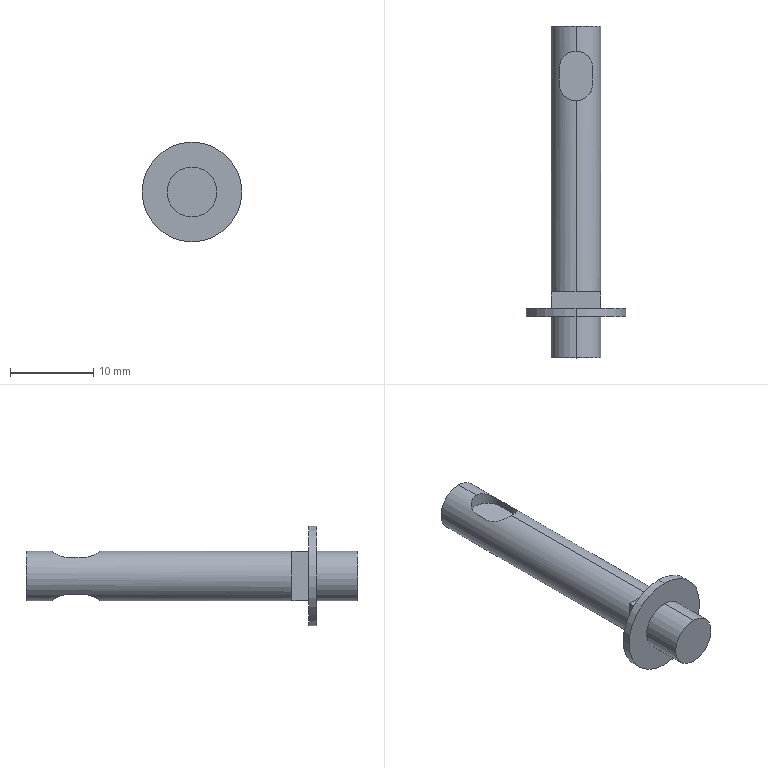Part | SolidWorks | features ICE 4, Revolution 1 | 1 solid | 28 faces | box 12 x 39.95 x 12 mm | volume 1172 mm3 | plane 18 | cylinder 10 | commonest cylinder face diameters 4 x4 6 x4 12 x2
STEP:
#1=CARTESIAN_POINT('',(0.,4.95,-3.));
#2=VERTEX_POINT('',#1);
#3=CARTESIAN_POINT('',(0.,4.95,3.));
#4=VERTEX_POINT('',#3);
#5=CARTESIAN_POINT('',(0.,4.95,0.));
#6=DIRECTION('',(0.,-1.,0.));
#7=DIRECTION('',(0.,0.,-1.));
#8=AXIS2_PLACEMENT_3D('',#5,#6,#7);
#9=CIRCLE('',#8,3.);
#10=EDGE_CURVE('',#2,#4,#9,.T.);
#11=ORIENTED_EDGE('',*,*,#10,.T.);
#12=CARTESIAN_POINT('',(0.,0.,3.));
#13=VERTEX_POINT('',#12);
#14=CARTESIAN_POINT('',(0.,-2.86,3.));
#15=DIRECTION('',(0.,-1.,0.));
#16=VECTOR('',#15,1000.);
#17=LINE('',#14,#16);
#18=EDGE_CURVE('',#4,#13,#17,.T.);
#19=ORIENTED_EDGE('',*,*,#18,.T.);
#20=CARTESIAN_POINT('',(0.,0.,-3.));
#21=VERTEX_POINT('',#20);
#22=CARTESIAN_POINT('',(0.,0.,0.));
#23=DIRECTION('',(0.,-1.,0.));
#24=DIRECTION('',(0.,0.,-1.));
#25=AXIS2_PLACEMENT_3D('',#22,#23,#24);
#26=CIRCLE('',#25,3.);
#27=EDGE_CURVE('',#21,#13,#26,.T.);
#28=ORIENTED_EDGE('',*,*,#27,.F.);
#29=CARTESIAN_POINT('',(0.,-2.86,-3.));
#30=DIRECTION('',(0.,-1.,0.));
#31=VECTOR('',#30,1000.);
#32=LINE('',#29,#31);
#33=EDGE_CURVE('',#2,#21,#32,.T.);
#34=ORIENTED_EDGE('',*,*,#33,.F.);
#35=EDGE_LOOP('',(#11,#19,#28,#34));
#36=FACE_OUTER_BOUND('',#35,.T.);
#37=CARTESIAN_POINT('',(0.,-2.86,0.));
#38=DIRECTION('',(0.,-1.,0.));
#39=DIRECTION('',(0.,0.,-1.));
#40=AXIS2_PLACEMENT_3D('',#37,#38,#39);
#41=CYLINDRICAL_SURFACE('',#40,3.);
#42=ADVANCED_FACE('',(#36),#41,.T.);
#43=CARTESIAN_POINT('',(0.,5.95,-6.));
#44=VERTEX_POINT('',#43);
#45=CARTESIAN_POINT('',(0.,5.95,6.));
#46=VERTEX_POINT('',#45);
#47=CARTESIAN_POINT('',(0.,5.95,0.));
#48=DIRECTION('',(0.,-1.,0.));
#49=DIRECTION('',(0.,0.,-1.));
#50=AXIS2_PLACEMENT_3D('',#47,#48,#49);
#51=CIRCLE('',#50,6.);
#52=EDGE_CURVE('',#44,#46,#51,.T.);
#53=ORIENTED_EDGE('',*,*,#52,.T.);
#54=CARTESIAN_POINT('',(0.,4.95,6.));
#55=VERTEX_POINT('',#54);
#56=CARTESIAN_POINT('',(0.,-2.86,6.));
#57=DIRECTION('',(0.,-1.,0.));
#58=VECTOR('',#57,1000.);
#59=LINE('',#56,#58);
#60=EDGE_CURVE('',#46,#55,#59,.T.);
#61=ORIENTED_EDGE('',*,*,#60,.T.);
#62=CARTESIAN_POINT('',(0.,4.95,-6.));
#63=VERTEX_POINT('',#62);
#64=CARTESIAN_POINT('',(0.,4.95,0.));
#65=DIRECTION('',(0.,-1.,0.));
#66=DIRECTION('',(0.,0.,-1.));
#67=AXIS2_PLACEMENT_3D('',#64,#65,#66);
#68=CIRCLE('',#67,6.);
#69=EDGE_CURVE('',#63,#55,#68,.T.);
#70=ORIENTED_EDGE('',*,*,#69,.F.);
#71=CARTESIAN_POINT('',(0.,-2.86,-6.));
#72=DIRECTION('',(0.,-1.,0.));
#73=VECTOR('',#72,1000.);
#74=LINE('',#71,#73);
#75=EDGE_CURVE('',#44,#63,#74,.T.);
#76=ORIENTED_EDGE('',*,*,#75,.F.);
#77=EDGE_LOOP('',(#53,#61,#70,#76));
#78=FACE_OUTER_BOUND('',#77,.T.);
#79=CARTESIAN_POINT('',(0.,-2.86,0.));
#80=DIRECTION('',(0.,-1.,0.));
#81=DIRECTION('',(0.,0.,-1.));
#82=AXIS2_PLACEMENT_3D('',#79,#80,#81);
#83=CYLINDRICAL_SURFACE('',#82,6.);
#84=ADVANCED_FACE('',(#78),#83,.T.);
#85=CARTESIAN_POINT('',(0.,39.95,3.));
#86=VERTEX_POINT('',#85);
#87=CARTESIAN_POINT('',(0.,39.95,-3.));
#88=VERTEX_POINT('',#87);
#89=CARTESIAN_POINT('',(0.,39.95,0.));
#90=DIRECTION('',(0.,1.,0.));
#91=DIRECTION('',(0.,0.,1.));
#92=AXIS2_PLACEMENT_3D('',#89,#90,#91);
#93=CIRCLE('',#92,3.);
#94=EDGE_CURVE('',#86,#88,#93,.T.);
#95=ORIENTED_EDGE('',*,*,#94,.F.);
#96=CARTESIAN_POINT('',(0.,36.95,3.));
#97=VERTEX_POINT('',#96);
#98=CARTESIAN_POINT('',(0.,39.95,3.));
#99=DIRECTION('',(0.,-1.,0.));
#100=VECTOR('',#99,1000.);
#101=LINE('',#98,#100);
#102=EDGE_CURVE('',#86,#97,#101,.T.);
#103=ORIENTED_EDGE('',*,*,#102,.T.);
#104=CARTESIAN_POINT('',(2.,34.95,2.236));
#105=VERTEX_POINT('',#104);
#106=CARTESIAN_POINT('',(0.,36.95,3.));
#107=CARTESIAN_POINT('',(0.1362,36.95,3.));
#108=CARTESIAN_POINT('',(0.2713,36.936,2.991));
#109=CARTESIAN_POINT('',(0.5335,36.882,2.955));
#110=CARTESIAN_POINT('',(0.6626,36.842,2.929));
#111=CARTESIAN_POINT('',(1.025,36.687,2.831));
#112=CARTESIAN_POINT('',(1.24,36.539,2.739));
#113=CARTESIAN_POINT('',(1.508,36.27,2.596));
#114=CARTESIAN_POINT('',(1.589,36.171,2.546));
#115=CARTESIAN_POINT('',(1.73,35.961,2.452));
#116=CARTESIAN_POINT('',(1.791,35.849,2.408));
#117=CARTESIAN_POINT('',(1.892,35.611,2.329));
#118=CARTESIAN_POINT('',(1.932,35.484,2.295));
#119=CARTESIAN_POINT('',(1.986,35.223,2.249));
#120=CARTESIAN_POINT('',(2.,35.087,2.236));
#121=CARTESIAN_POINT('',(2.,34.95,2.236));
#122=B_SPLINE_CURVE_WITH_KNOTS('',3,(#106,#107,#108,#109,#110,#111,#112,#113,#114,#115,#116,#117,#118,#119,#120,#121),.UNSPECIFIED.,.F.,.F.,(4,2,2,2,2,2,2,4),(0.003235,0.003638,0.004041,0.004847,0.00525,0.005653,0.006056,0.006459),.UNSPECIFIED.);
#123=EDGE_CURVE('',#97,#105,#122,.T.);
#124=ORIENTED_EDGE('',*,*,#123,.T.);
#125=CARTESIAN_POINT('',(2.,32.95,2.236));
#126=VERTEX_POINT('',#125);
#127=CARTESIAN_POINT('',(2.,39.95,2.236));
#128=DIRECTION('',(0.,-1.,0.));
#129=VECTOR('',#128,1000.);
#130=LINE('',#127,#129);
#131=EDGE_CURVE('',#105,#126,#130,.T.);
#132=ORIENTED_EDGE('',*,*,#131,.T.);
#133=CARTESIAN_POINT('',(0.,30.95,3.));
#134=VERTEX_POINT('',#133);
#135=CARTESIAN_POINT('',(2.,32.95,2.236));
#136=CARTESIAN_POINT('',(2.,32.813,2.236));
#137=CARTESIAN_POINT('',(1.986,32.679,2.249));
#138=CARTESIAN_POINT('',(1.933,32.418,2.295));
#139=CARTESIAN_POINT('',(1.892,32.29,2.329));
#140=CARTESIAN_POINT('',(1.741,31.932,2.447));
#141=CARTESIAN_POINT('',(1.596,31.719,2.548));
#142=CARTESIAN_POINT('',(1.328,31.449,2.692));
#143=CARTESIAN_POINT('',(1.228,31.366,2.739));
#144=CARTESIAN_POINT('',(1.016,31.223,2.825));
#145=CARTESIAN_POINT('',(0.9033,31.161,2.864));
#146=CARTESIAN_POINT('',(0.6618,31.058,2.929));
#147=CARTESIAN_POINT('',(0.5321,31.017,2.955));
#148=CARTESIAN_POINT('',(0.2704,30.964,2.991));
#149=CARTESIAN_POINT('',(0.1367,30.95,3.));
#150=CARTESIAN_POINT('',(0.,30.95,3.));
#151=B_SPLINE_CURVE_WITH_KNOTS('',3,(#135,#136,#137,#138,#139,#140,#141,#142,#143,#144,#145,#146,#147,#148,#149,#150),.UNSPECIFIED.,.F.,.F.,(4,2,2,2,2,2,2,4),(0.,0.0004044,0.0008088,0.001618,0.002022,0.002426,0.002831,0.003235),.UNSPECIFIED.);
#152=EDGE_CURVE('',#126,#134,#151,.T.);
#153=ORIENTED_EDGE('',*,*,#152,.T.);
#154=CARTESIAN_POINT('',(0.,7.95,3.));
#155=VERTEX_POINT('',#154);
#156=CARTESIAN_POINT('',(0.,39.95,3.));
#157=DIRECTION('',(0.,-1.,0.));
#158=VECTOR('',#157,1000.);
#159=LINE('',#156,#158);
#160=EDGE_CURVE('',#134,#155,#159,.T.);
#161=ORIENTED_EDGE('',*,*,#160,.T.);
#162=CARTESIAN_POINT('',(3.,7.95,0.));
#163=VERTEX_POINT('',#162);
#164=CARTESIAN_POINT('',(0.,7.95,0.));
#165=DIRECTION('',(0.,1.,0.));
#166=DIRECTION('',(0.,0.,1.));
#167=AXIS2_PLACEMENT_3D('',#164,#165,#166);
#168=CIRCLE('',#167,3.);
#169=EDGE_CURVE('',#155,#163,#168,.T.);
#170=ORIENTED_EDGE('',*,*,#169,.T.);
#171=CARTESIAN_POINT('',(0.,7.95,-3.));
#172=VERTEX_POINT('',#171);
#173=CARTESIAN_POINT('',(0.,7.95,0.));
#174=DIRECTION('',(0.,1.,0.));
#175=DIRECTION('',(0.,0.,1.));
#176=AXIS2_PLACEMENT_3D('',#173,#174,#175);
#177=CIRCLE('',#176,3.);
#178=EDGE_CURVE('',#163,#172,#177,.T.);
#179=ORIENTED_EDGE('',*,*,#178,.T.);
#180=CARTESIAN_POINT('',(0.,30.95,-3.));
#181=VERTEX_POINT('',#180);
#182=CARTESIAN_POINT('',(0.,39.95,-3.));
#183=DIRECTION('',(0.,-1.,0.));
#184=VECTOR('',#183,1000.);
#185=LINE('',#182,#184);
#186=EDGE_CURVE('',#181,#172,#185,.T.);
#187=ORIENTED_EDGE('',*,*,#186,.F.);
#188=CARTESIAN_POINT('',(2.,32.95,-2.236));
#189=VERTEX_POINT('',#188);
#190=CARTESIAN_POINT('',(2.,32.95,-2.236));
#191=CARTESIAN_POINT('',(2.,32.813,-2.236));
#192=CARTESIAN_POINT('',(1.986,32.679,-2.249));
#193=CARTESIAN_POINT('',(1.933,32.418,-2.295));
#194=CARTESIAN_POINT('',(1.892,32.29,-2.329));
#195=CARTESIAN_POINT('',(1.741,31.932,-2.447));
#196=CARTESIAN_POINT('',(1.596,31.719,-2.548));
#197=CARTESIAN_POINT('',(1.328,31.449,-2.692));
#198=CARTESIAN_POINT('',(1.228,31.366,-2.739));
#199=CARTESIAN_POINT('',(1.016,31.223,-2.825));
#200=CARTESIAN_POINT('',(0.9033,31.161,-2.864));
#201=CARTESIAN_POINT('',(0.6618,31.058,-2.929));
#202=CARTESIAN_POINT('',(0.5321,31.017,-2.955));
#203=CARTESIAN_POINT('',(0.2704,30.964,-2.991));
#204=CARTESIAN_POINT('',(0.1367,30.95,-3.));
#205=CARTESIAN_POINT('',(0.,30.95,-3.));
#206=B_SPLINE_CURVE_WITH_KNOTS('',3,(#190,#191,#192,#193,#194,#195,#196,#197,#198,#199,#200,#201,#202,#203,#204,#205),.UNSPECIFIED.,.F.,.F.,(4,2,2,2,2,2,2,4),(0.,0.0004044,0.0008088,0.001618,0.002022,0.002426,0.002831,0.003235),.UNSPECIFIED.);
#207=EDGE_CURVE('',#189,#181,#206,.T.);
#208=ORIENTED_EDGE('',*,*,#207,.F.);
#209=CARTESIAN_POINT('',(2.,34.95,-2.236));
#210=VERTEX_POINT('',#209);
#211=CARTESIAN_POINT('',(2.,39.95,-2.236));
#212=DIRECTION('',(0.,-1.,0.));
#213=VECTOR('',#212,1000.);
#214=LINE('',#211,#213);
#215=EDGE_CURVE('',#210,#189,#214,.T.);
#216=ORIENTED_EDGE('',*,*,#215,.F.);
#217=CARTESIAN_POINT('',(0.,36.95,-3.));
#218=VERTEX_POINT('',#217);
#219=CARTESIAN_POINT('',(0.,36.95,-3.));
#220=CARTESIAN_POINT('',(0.1362,36.95,-3.));
#221=CARTESIAN_POINT('',(0.2713,36.936,-2.991));
#222=CARTESIAN_POINT('',(0.5335,36.882,-2.955));
#223=CARTESIAN_POINT('',(0.6626,36.842,-2.929));
#224=CARTESIAN_POINT('',(1.025,36.687,-2.831));
#225=CARTESIAN_POINT('',(1.24,36.539,-2.739));
#226=CARTESIAN_POINT('',(1.508,36.27,-2.596));
#227=CARTESIAN_POINT('',(1.589,36.171,-2.546));
#228=CARTESIAN_POINT('',(1.73,35.961,-2.452));
#229=CARTESIAN_POINT('',(1.791,35.849,-2.408));
#230=CARTESIAN_POINT('',(1.892,35.611,-2.329));
#231=CARTESIAN_POINT('',(1.932,35.484,-2.295));
#232=CARTESIAN_POINT('',(1.986,35.223,-2.249));
#233=CARTESIAN_POINT('',(2.,35.087,-2.236));
#234=CARTESIAN_POINT('',(2.,34.95,-2.236));
#235=B_SPLINE_CURVE_WITH_KNOTS('',3,(#219,#220,#221,#222,#223,#224,#225,#226,#227,#228,#229,#230,#231,#232,#233,#234),.UNSPECIFIED.,.F.,.F.,(4,2,2,2,2,2,2,4),(0.003235,0.003638,0.004041,0.004847,0.00525,0.005653,0.006056,0.006459),.UNSPECIFIED.);
#236=EDGE_CURVE('',#218,#210,#235,.T.);
#237=ORIENTED_EDGE('',*,*,#236,.F.);
#238=CARTESIAN_POINT('',(0.,39.95,-3.));
#239=DIRECTION('',(0.,-1.,0.));
#240=VECTOR('',#239,1000.);
#241=LINE('',#238,#240);
#242=EDGE_CURVE('',#88,#218,#241,.T.);
#243=ORIENTED_EDGE('',*,*,#242,.F.);
#244=EDGE_LOOP('',(#95,#103,#124,#132,#153,#161,#170,#179,#187,#208,#216,#237,#243));
#245=FACE_OUTER_BOUND('',#244,.T.);
#246=CARTESIAN_POINT('',(0.,39.95,0.));
#247=DIRECTION('',(0.,-1.,0.));
#248=DIRECTION('',(0.,0.,-1.));
#249=AXIS2_PLACEMENT_3D('',#246,#247,#248);
#250=CYLINDRICAL_SURFACE('',#249,3.);
#251=ADVANCED_FACE('',(#245),#250,.T.);
#252=ORIENTED_EDGE('',*,*,#102,.F.);
#253=CARTESIAN_POINT('',(0.,39.95,0.));
#254=DIRECTION('',(0.,1.,0.));
#255=DIRECTION('',(0.,0.,1.));
#256=AXIS2_PLACEMENT_3D('',#253,#254,#255);
#257=CIRCLE('',#256,3.);
#258=EDGE_CURVE('',#88,#86,#257,.T.);
#259=ORIENTED_EDGE('',*,*,#258,.F.);
#260=ORIENTED_EDGE('',*,*,#242,.T.);
#261=CARTESIAN_POINT('',(-2.,34.95,-2.236));
#262=VERTEX_POINT('',#261);
#263=CARTESIAN_POINT('',(-2.,34.95,-2.236));
#264=CARTESIAN_POINT('',(-2.,35.087,-2.236));
#265=CARTESIAN_POINT('',(-1.986,35.221,-2.249));
#266=CARTESIAN_POINT('',(-1.933,35.482,-2.295));
#267=CARTESIAN_POINT('',(-1.892,35.61,-2.329));
#268=CARTESIAN_POINT('',(-1.741,35.968,-2.447));
#269=CARTESIAN_POINT('',(-1.596,36.181,-2.548));
#270=CARTESIAN_POINT('',(-1.328,36.451,-2.692));
#271=CARTESIAN_POINT('',(-1.228,36.534,-2.739));
#272=CARTESIAN_POINT('',(-1.016,36.677,-2.825));
#273=CARTESIAN_POINT('',(-0.9033,36.739,-2.864));
#274=CARTESIAN_POINT('',(-0.6618,36.842,-2.929));
#275=CARTESIAN_POINT('',(-0.5321,36.883,-2.955));
#276=CARTESIAN_POINT('',(-0.2704,36.936,-2.991));
#277=CARTESIAN_POINT('',(-0.1367,36.95,-3.));
#278=CARTESIAN_POINT('',(0.,36.95,-3.));
#279=B_SPLINE_CURVE_WITH_KNOTS('',3,(#263,#264,#265,#266,#267,#268,#269,#270,#271,#272,#273,#274,#275,#276,#277,#278),.UNSPECIFIED.,.F.,.F.,(4,2,2,2,2,2,2,4),(0.,0.0004044,0.0008088,0.001618,0.002022,0.002426,0.002831,0.003235),.UNSPECIFIED.);
#280=EDGE_CURVE('',#262,#218,#279,.T.);
#281=ORIENTED_EDGE('',*,*,#280,.F.);
#282=CARTESIAN_POINT('',(-2.,32.95,-2.236));
#283=VERTEX_POINT('',#282);
#284=CARTESIAN_POINT('',(-2.,39.95,-2.236));
#285=DIRECTION('',(0.,1.,0.));
#286=VECTOR('',#285,1000.);
#287=LINE('',#284,#286);
#288=EDGE_CURVE('',#283,#262,#287,.T.);
#289=ORIENTED_EDGE('',*,*,#288,.F.);
#290=CARTESIAN_POINT('',(0.,30.95,-3.));
#291=CARTESIAN_POINT('',(-0.1362,30.95,-3.));
#292=CARTESIAN_POINT('',(-0.2713,30.964,-2.991));
#293=CARTESIAN_POINT('',(-0.5335,31.018,-2.955));
#294=CARTESIAN_POINT('',(-0.6626,31.058,-2.929));
#295=CARTESIAN_POINT('',(-1.025,31.213,-2.831));
#296=CARTESIAN_POINT('',(-1.24,31.361,-2.739));
#297=CARTESIAN_POINT('',(-1.508,31.63,-2.596));
#298=CARTESIAN_POINT('',(-1.589,31.729,-2.546));
#299=CARTESIAN_POINT('',(-1.73,31.939,-2.452));
#300=CARTESIAN_POINT('',(-1.791,32.051,-2.408));
#301=CARTESIAN_POINT('',(-1.892,32.289,-2.329));
#302=CARTESIAN_POINT('',(-1.932,32.416,-2.295));
#303=CARTESIAN_POINT('',(-1.986,32.677,-2.249));
#304=CARTESIAN_POINT('',(-2.,32.813,-2.236));
#305=CARTESIAN_POINT('',(-2.,32.95,-2.236));
#306=B_SPLINE_CURVE_WITH_KNOTS('',3,(#290,#291,#292,#293,#294,#295,#296,#297,#298,#299,#300,#301,#302,#303,#304,#305),.UNSPECIFIED.,.F.,.F.,(4,2,2,2,2,2,2,4),(0.003235,0.003638,0.004041,0.004847,0.00525,0.005653,0.006056,0.006459),.UNSPECIFIED.);
#307=EDGE_CURVE('',#181,#283,#306,.T.);
#308=ORIENTED_EDGE('',*,*,#307,.F.);
#309=ORIENTED_EDGE('',*,*,#186,.T.);
#310=CARTESIAN_POINT('',(-3.,7.95,0.));
#311=VERTEX_POINT('',#310);
#312=CARTESIAN_POINT('',(0.,7.95,0.));
#313=DIRECTION('',(0.,1.,0.));
#314=DIRECTION('',(0.,0.,1.));
#315=AXIS2_PLACEMENT_3D('',#312,#313,#314);
#316=CIRCLE('',#315,3.);
#317=EDGE_CURVE('',#172,#311,#316,.T.);
#318=ORIENTED_EDGE('',*,*,#317,.T.);
#319=CARTESIAN_POINT('',(0.,7.95,0.));
#320=DIRECTION('',(0.,1.,0.));
#321=DIRECTION('',(0.,0.,1.));
#322=AXIS2_PLACEMENT_3D('',#319,#320,#321);
#323=CIRCLE('',#322,3.);
#324=EDGE_CURVE('',#311,#155,#323,.T.);
#325=ORIENTED_EDGE('',*,*,#324,.T.);
#326=ORIENTED_EDGE('',*,*,#160,.F.);
#327=CARTESIAN_POINT('',(-2.,32.95,2.236));
#328=VERTEX_POINT('',#327);
#329=CARTESIAN_POINT('',(0.,30.95,3.));
#330=CARTESIAN_POINT('',(-0.1362,30.95,3.));
#331=CARTESIAN_POINT('',(-0.2713,30.964,2.991));
#332=CARTESIAN_POINT('',(-0.5335,31.018,2.955));
#333=CARTESIAN_POINT('',(-0.6626,31.058,2.929));
#334=CARTESIAN_POINT('',(-1.025,31.213,2.831));
#335=CARTESIAN_POINT('',(-1.24,31.361,2.739));
#336=CARTESIAN_POINT('',(-1.508,31.63,2.596));
#337=CARTESIAN_POINT('',(-1.589,31.729,2.546));
#338=CARTESIAN_POINT('',(-1.73,31.939,2.452));
#339=CARTESIAN_POINT('',(-1.791,32.051,2.408));
#340=CARTESIAN_POINT('',(-1.892,32.289,2.329));
#341=CARTESIAN_POINT('',(-1.932,32.416,2.295));
#342=CARTESIAN_POINT('',(-1.986,32.677,2.249));
#343=CARTESIAN_POINT('',(-2.,32.813,2.236));
#344=CARTESIAN_POINT('',(-2.,32.95,2.236));
#345=B_SPLINE_CURVE_WITH_KNOTS('',3,(#329,#330,#331,#332,#333,#334,#335,#336,#337,#338,#339,#340,#341,#342,#343,#344),.UNSPECIFIED.,.F.,.F.,(4,2,2,2,2,2,2,4),(0.003235,0.003638,0.004041,0.004847,0.00525,0.005653,0.006056,0.006459),.UNSPECIFIED.);
#346=EDGE_CURVE('',#134,#328,#345,.T.);
#347=ORIENTED_EDGE('',*,*,#346,.T.);
#348=CARTESIAN_POINT('',(-2.,34.95,2.236));
#349=VERTEX_POINT('',#348);
#350=CARTESIAN_POINT('',(-2.,39.95,2.236));
#351=DIRECTION('',(0.,1.,0.));
#352=VECTOR('',#351,1000.);
#353=LINE('',#350,#352);
#354=EDGE_CURVE('',#328,#349,#353,.T.);
#355=ORIENTED_EDGE('',*,*,#354,.T.);
#356=CARTESIAN_POINT('',(-2.,34.95,2.236));
#357=CARTESIAN_POINT('',(-2.,35.087,2.236));
#358=CARTESIAN_POINT('',(-1.986,35.221,2.249));
#359=CARTESIAN_POINT('',(-1.933,35.482,2.295));
#360=CARTESIAN_POINT('',(-1.892,35.61,2.329));
#361=CARTESIAN_POINT('',(-1.741,35.968,2.447));
#362=CARTESIAN_POINT('',(-1.596,36.181,2.548));
#363=CARTESIAN_POINT('',(-1.328,36.451,2.692));
#364=CARTESIAN_POINT('',(-1.228,36.534,2.739));
#365=CARTESIAN_POINT('',(-1.016,36.677,2.825));
#366=CARTESIAN_POINT('',(-0.9033,36.739,2.864));
#367=CARTESIAN_POINT('',(-0.6618,36.842,2.929));
#368=CARTESIAN_POINT('',(-0.5321,36.883,2.955));
#369=CARTESIAN_POINT('',(-0.2704,36.936,2.991));
#370=CARTESIAN_POINT('',(-0.1367,36.95,3.));
#371=CARTESIAN_POINT('',(0.,36.95,3.));
#372=B_SPLINE_CURVE_WITH_KNOTS('',3,(#356,#357,#358,#359,#360,#361,#362,#363,#364,#365,#366,#367,#368,#369,#370,#371),.UNSPECIFIED.,.F.,.F.,(4,2,2,2,2,2,2,4),(0.,0.0004044,0.0008088,0.001618,0.002022,0.002426,0.002831,0.003235),.UNSPECIFIED.);
#373=EDGE_CURVE('',#349,#97,#372,.T.);
#374=ORIENTED_EDGE('',*,*,#373,.T.);
#375=EDGE_LOOP('',(#252,#259,#260,#281,#289,#308,#309,#318,#325,#326,#347,#355,#374));
#376=FACE_OUTER_BOUND('',#375,.T.);
#377=CARTESIAN_POINT('',(0.,39.95,0.));
#378=DIRECTION('',(0.,-1.,0.));
#379=DIRECTION('',(0.,0.,-1.));
#380=AXIS2_PLACEMENT_3D('',#377,#378,#379);
#381=CYLINDRICAL_SURFACE('',#380,3.);
#382=ADVANCED_FACE('',(#376),#381,.T.);
#383=ORIENTED_EDGE('',*,*,#169,.F.);
#384=CARTESIAN_POINT('',(3.,7.95,3.));
#385=VERTEX_POINT('',#384);
#386=CARTESIAN_POINT('',(-3.,7.95,3.));
#387=DIRECTION('',(1.,0.,0.));
#388=VECTOR('',#387,1000.);
#389=LINE('',#386,#388);
#390=EDGE_CURVE('',#155,#385,#389,.T.);
#391=ORIENTED_EDGE('',*,*,#390,.T.);
#392=CARTESIAN_POINT('',(3.,7.95,-3.));
#393=DIRECTION('',(0.,0.,-1.));
#394=VECTOR('',#393,1000.);
#395=LINE('',#392,#394);
#396=EDGE_CURVE('',#385,#163,#395,.T.);
#397=ORIENTED_EDGE('',*,*,#396,.T.);
#398=EDGE_LOOP('',(#383,#391,#397));
#399=FACE_OUTER_BOUND('',#398,.T.);
#400=CARTESIAN_POINT('',(0.,7.95,0.));
#401=DIRECTION('',(0.,1.,0.));
#402=DIRECTION('',(0.,0.,1.));
#403=AXIS2_PLACEMENT_3D('',#400,#401,#402);
#404=PLANE('',#403);
#405=ADVANCED_FACE('',(#399),#404,.T.);
#406=ORIENTED_EDGE('',*,*,#178,.F.);
#407=CARTESIAN_POINT('',(3.,7.95,-3.));
#408=VERTEX_POINT('',#407);
#409=CARTESIAN_POINT('',(3.,7.95,-3.));
#410=DIRECTION('',(0.,0.,-1.));
#411=VECTOR('',#410,1000.);
#412=LINE('',#409,#411);
#413=EDGE_CURVE('',#163,#408,#412,.T.);
#414=ORIENTED_EDGE('',*,*,#413,.T.);
#415=CARTESIAN_POINT('',(-3.,7.95,-3.));
#416=DIRECTION('',(-1.,0.,0.));
#417=VECTOR('',#416,1000.);
#418=LINE('',#415,#417);
#419=EDGE_CURVE('',#408,#172,#418,.T.);
#420=ORIENTED_EDGE('',*,*,#419,.T.);
#421=EDGE_LOOP('',(#406,#414,#420));
#422=FACE_OUTER_BOUND('',#421,.T.);
#423=CARTESIAN_POINT('',(0.,7.95,0.));
#424=DIRECTION('',(0.,1.,0.));
#425=DIRECTION('',(0.,0.,1.));
#426=AXIS2_PLACEMENT_3D('',#423,#424,#425);
#427=PLANE('',#426);
#428=ADVANCED_FACE('',(#422),#427,.T.);
#429=ORIENTED_EDGE('',*,*,#317,.F.);
#430=CARTESIAN_POINT('',(-3.,7.95,-3.));
#431=VERTEX_POINT('',#430);
#432=CARTESIAN_POINT('',(-3.,7.95,-3.));
#433=DIRECTION('',(-1.,0.,0.));
#434=VECTOR('',#433,1000.);
#435=LINE('',#432,#434);
#436=EDGE_CURVE('',#172,#431,#435,.T.);
#437=ORIENTED_EDGE('',*,*,#436,.T.);
#438=CARTESIAN_POINT('',(-3.,7.95,-3.));
#439=DIRECTION('',(0.,0.,1.));
#440=VECTOR('',#439,1000.);
#441=LINE('',#438,#440);
#442=EDGE_CURVE('',#431,#311,#441,.T.);
#443=ORIENTED_EDGE('',*,*,#442,.T.);
#444=EDGE_LOOP('',(#429,#437,#443));
#445=FACE_OUTER_BOUND('',#444,.T.);
#446=CARTESIAN_POINT('',(0.,7.95,0.));
#447=DIRECTION('',(0.,1.,0.));
#448=DIRECTION('',(0.,0.,1.));
#449=AXIS2_PLACEMENT_3D('',#446,#447,#448);
#450=PLANE('',#449);
#451=ADVANCED_FACE('',(#445),#450,.T.);
#452=CARTESIAN_POINT('',(3.,5.95,3.));
#453=VERTEX_POINT('',#452);
#454=CARTESIAN_POINT('',(3.,5.95,-3.));
#455=VERTEX_POINT('',#454);
#456=CARTESIAN_POINT('',(3.,5.95,-3.));
#457=DIRECTION('',(0.,0.,-1.));
#458=VECTOR('',#457,1000.);
#459=LINE('',#456,#458);
#460=EDGE_CURVE('',#453,#455,#459,.T.);
#461=ORIENTED_EDGE('',*,*,#460,.F.);
#462=CARTESIAN_POINT('',(-3.,5.95,3.));
#463=VERTEX_POINT('',#462);
#464=CARTESIAN_POINT('',(-3.,5.95,3.));
#465=DIRECTION('',(1.,0.,0.));
#466=VECTOR('',#465,1000.);
#467=LINE('',#464,#466);
#468=EDGE_CURVE('',#463,#453,#467,.T.);
#469=ORIENTED_EDGE('',*,*,#468,.F.);
#470=CARTESIAN_POINT('',(-3.,5.95,-3.));
#471=VERTEX_POINT('',#470);
#472=CARTESIAN_POINT('',(-3.,5.95,-3.));
#473=DIRECTION('',(0.,0.,1.));
#474=VECTOR('',#473,1000.);
#475=LINE('',#472,#474);
#476=EDGE_CURVE('',#471,#463,#475,.T.);
#477=ORIENTED_EDGE('',*,*,#476,.F.);
#478=CARTESIAN_POINT('',(-3.,5.95,-3.));
#479=DIRECTION('',(-1.,0.,0.));
#480=VECTOR('',#479,1000.);
#481=LINE('',#478,#480);
#482=EDGE_CURVE('',#455,#471,#481,.T.);
#483=ORIENTED_EDGE('',*,*,#482,.F.);
#484=EDGE_LOOP('',(#461,#469,#477,#483));
#485=FACE_BOUND('',#484,.T.);
#486=ORIENTED_EDGE('',*,*,#52,.F.);
#487=CARTESIAN_POINT('',(0.,5.95,0.));
#488=DIRECTION('',(0.,-1.,0.));
#489=DIRECTION('',(0.,0.,-1.));
#490=AXIS2_PLACEMENT_3D('',#487,#488,#489);
#491=CIRCLE('',#490,6.);
#492=EDGE_CURVE('',#46,#44,#491,.T.);
#493=ORIENTED_EDGE('',*,*,#492,.F.);
#494=EDGE_LOOP('',(#486,#493));
#495=FACE_OUTER_BOUND('',#494,.T.);
#496=CARTESIAN_POINT('',(0.,5.95,0.));
#497=DIRECTION('',(0.,1.,0.));
#498=DIRECTION('',(0.,0.,1.));
#499=AXIS2_PLACEMENT_3D('',#496,#497,#498);
#500=PLANE('',#499);
#501=ADVANCED_FACE('',(#485,#495),#500,.T.);
#502=ORIENTED_EDGE('',*,*,#60,.F.);
#503=ORIENTED_EDGE('',*,*,#492,.T.);
#504=ORIENTED_EDGE('',*,*,#75,.T.);
#505=CARTESIAN_POINT('',(0.,4.95,0.));
#506=DIRECTION('',(0.,-1.,0.));
#507=DIRECTION('',(0.,0.,-1.));
#508=AXIS2_PLACEMENT_3D('',#505,#506,#507);
#509=CIRCLE('',#508,6.);
#510=EDGE_CURVE('',#55,#63,#509,.T.);
#511=ORIENTED_EDGE('',*,*,#510,.F.);
#512=EDGE_LOOP('',(#502,#503,#504,#511));
#513=FACE_OUTER_BOUND('',#512,.T.);
#514=CARTESIAN_POINT('',(0.,-2.86,0.));
#515=DIRECTION('',(0.,-1.,0.));
#516=DIRECTION('',(0.,0.,-1.));
#517=AXIS2_PLACEMENT_3D('',#514,#515,#516);
#518=CYLINDRICAL_SURFACE('',#517,6.);
#519=ADVANCED_FACE('',(#513),#518,.T.);
#520=ORIENTED_EDGE('',*,*,#69,.T.);
#521=ORIENTED_EDGE('',*,*,#510,.T.);
#522=EDGE_LOOP('',(#520,#521));
#523=FACE_OUTER_BOUND('',#522,.T.);
#524=ORIENTED_EDGE('',*,*,#10,.F.);
#525=CARTESIAN_POINT('',(0.,4.95,0.));
#526=DIRECTION('',(0.,-1.,0.));
#527=DIRECTION('',(0.,0.,-1.));
#528=AXIS2_PLACEMENT_3D('',#525,#526,#527);
#529=CIRCLE('',#528,3.);
#530=EDGE_CURVE('',#4,#2,#529,.T.);
#531=ORIENTED_EDGE('',*,*,#530,.F.);
#532=EDGE_LOOP('',(#524,#531));
#533=FACE_BOUND('',#532,.T.);
#534=CARTESIAN_POINT('',(6.,4.95,0.));
#535=DIRECTION('',(0.,-1.,0.));
#536=DIRECTION('',(0.,0.,-1.));
#537=AXIS2_PLACEMENT_3D('',#534,#535,#536);
#538=PLANE('',#537);
#539=ADVANCED_FACE('',(#523,#533),#538,.T.);
#540=ORIENTED_EDGE('',*,*,#18,.F.);
#541=ORIENTED_EDGE('',*,*,#530,.T.);
#542=ORIENTED_EDGE('',*,*,#33,.T.);
#543=CARTESIAN_POINT('',(0.,0.,0.));
#544=DIRECTION('',(0.,-1.,0.));
#545=DIRECTION('',(0.,0.,-1.));
#546=AXIS2_PLACEMENT_3D('',#543,#544,#545);
#547=CIRCLE('',#546,3.);
#548=EDGE_CURVE('',#13,#21,#547,.T.);
#549=ORIENTED_EDGE('',*,*,#548,.F.);
#550=EDGE_LOOP('',(#540,#541,#542,#549));
#551=FACE_OUTER_BOUND('',#550,.T.);
#552=CARTESIAN_POINT('',(0.,-2.86,0.));
#553=DIRECTION('',(0.,-1.,0.));
#554=DIRECTION('',(0.,0.,-1.));
#555=AXIS2_PLACEMENT_3D('',#552,#553,#554);
#556=CYLINDRICAL_SURFACE('',#555,3.);
#557=ADVANCED_FACE('',(#551),#556,.T.);
#558=ORIENTED_EDGE('',*,*,#27,.T.);
#559=ORIENTED_EDGE('',*,*,#548,.T.);
#560=EDGE_LOOP('',(#558,#559));
#561=FACE_OUTER_BOUND('',#560,.T.);
#562=CARTESIAN_POINT('',(0.,0.,0.));
#563=DIRECTION('',(0.,-1.,0.));
#564=DIRECTION('',(0.,0.,-1.));
#565=AXIS2_PLACEMENT_3D('',#562,#563,#564);
#566=PLANE('',#565);
#567=ADVANCED_FACE('',(#561),#566,.T.);
#568=ORIENTED_EDGE('',*,*,#460,.T.);
#569=CARTESIAN_POINT('',(3.,7.95,-3.));
#570=DIRECTION('',(0.,-1.,0.));
#571=VECTOR('',#570,1000.);
#572=LINE('',#569,#571);
#573=EDGE_CURVE('',#408,#455,#572,.T.);
#574=ORIENTED_EDGE('',*,*,#573,.F.);
#575=ORIENTED_EDGE('',*,*,#413,.F.);
#576=ORIENTED_EDGE('',*,*,#396,.F.);
#577=CARTESIAN_POINT('',(3.,7.95,3.));
#578=DIRECTION('',(0.,-1.,0.));
#579=VECTOR('',#578,1000.);
#580=LINE('',#577,#579);
#581=EDGE_CURVE('',#385,#453,#580,.T.);
#582=ORIENTED_EDGE('',*,*,#581,.T.);
#583=EDGE_LOOP('',(#568,#574,#575,#576,#582));
#584=FACE_OUTER_BOUND('',#583,.T.);
#585=CARTESIAN_POINT('',(3.,7.95,-3.));
#586=DIRECTION('',(-1.,0.,0.));
#587=DIRECTION('',(0.,0.,1.));
#588=AXIS2_PLACEMENT_3D('',#585,#586,#587);
#589=PLANE('',#588);
#590=ADVANCED_FACE('',(#584),#589,.F.);
#591=ORIENTED_EDGE('',*,*,#482,.T.);
#592=CARTESIAN_POINT('',(-3.,7.95,-3.));
#593=DIRECTION('',(0.,-1.,0.));
#594=VECTOR('',#593,1000.);
#595=LINE('',#592,#594);
#596=EDGE_CURVE('',#431,#471,#595,.T.);
#597=ORIENTED_EDGE('',*,*,#596,.F.);
#598=ORIENTED_EDGE('',*,*,#436,.F.);
#599=ORIENTED_EDGE('',*,*,#419,.F.);
#600=ORIENTED_EDGE('',*,*,#573,.T.);
#601=EDGE_LOOP('',(#591,#597,#598,#599,#600));
#602=FACE_OUTER_BOUND('',#601,.T.);
#603=CARTESIAN_POINT('',(-3.,7.95,-3.));
#604=DIRECTION('',(0.,0.,1.));
#605=DIRECTION('',(1.,0.,0.));
#606=AXIS2_PLACEMENT_3D('',#603,#604,#605);
#607=PLANE('',#606);
#608=ADVANCED_FACE('',(#602),#607,.F.);
#609=ORIENTED_EDGE('',*,*,#476,.T.);
#610=CARTESIAN_POINT('',(-3.,7.95,3.));
#611=VERTEX_POINT('',#610);
#612=CARTESIAN_POINT('',(-3.,7.95,3.));
#613=DIRECTION('',(0.,-1.,0.));
#614=VECTOR('',#613,1000.);
#615=LINE('',#612,#614);
#616=EDGE_CURVE('',#611,#463,#615,.T.);
#617=ORIENTED_EDGE('',*,*,#616,.F.);
#618=CARTESIAN_POINT('',(-3.,7.95,-3.));
#619=DIRECTION('',(0.,0.,1.));
#620=VECTOR('',#619,1000.);
#621=LINE('',#618,#620);
#622=EDGE_CURVE('',#311,#611,#621,.T.);
#623=ORIENTED_EDGE('',*,*,#622,.F.);
#624=ORIENTED_EDGE('',*,*,#442,.F.);
#625=ORIENTED_EDGE('',*,*,#596,.T.);
#626=EDGE_LOOP('',(#609,#617,#623,#624,#625));
#627=FACE_OUTER_BOUND('',#626,.T.);
#628=CARTESIAN_POINT('',(-3.,7.95,-3.));
#629=DIRECTION('',(1.,0.,0.));
#630=DIRECTION('',(0.,0.,-1.));
#631=AXIS2_PLACEMENT_3D('',#628,#629,#630);
#632=PLANE('',#631);
#633=ADVANCED_FACE('',(#627),#632,.F.);
#634=ORIENTED_EDGE('',*,*,#468,.T.);
#635=ORIENTED_EDGE('',*,*,#581,.F.);
#636=ORIENTED_EDGE('',*,*,#390,.F.);
#637=CARTESIAN_POINT('',(-3.,7.95,3.));
#638=DIRECTION('',(1.,0.,0.));
#639=VECTOR('',#638,1000.);
#640=LINE('',#637,#639);
#641=EDGE_CURVE('',#611,#155,#640,.T.);
#642=ORIENTED_EDGE('',*,*,#641,.F.);
#643=ORIENTED_EDGE('',*,*,#616,.T.);
#644=EDGE_LOOP('',(#634,#635,#636,#642,#643));
#645=FACE_OUTER_BOUND('',#644,.T.);
#646=CARTESIAN_POINT('',(-3.,7.95,3.));
#647=DIRECTION('',(0.,0.,-1.));
#648=DIRECTION('',(-1.,0.,0.));
#649=AXIS2_PLACEMENT_3D('',#646,#647,#648);
#650=PLANE('',#649);
#651=ADVANCED_FACE('',(#645),#650,.F.);
#652=ORIENTED_EDGE('',*,*,#324,.F.);
#653=ORIENTED_EDGE('',*,*,#622,.T.);
#654=ORIENTED_EDGE('',*,*,#641,.T.);
#655=EDGE_LOOP('',(#652,#653,#654));
#656=FACE_OUTER_BOUND('',#655,.T.);
#657=CARTESIAN_POINT('',(0.,7.95,0.));
#658=DIRECTION('',(0.,1.,0.));
#659=DIRECTION('',(0.,0.,1.));
#660=AXIS2_PLACEMENT_3D('',#657,#658,#659);
#661=PLANE('',#660);
#662=ADVANCED_FACE('',(#656),#661,.T.);
#663=ORIENTED_EDGE('',*,*,#258,.T.);
#664=ORIENTED_EDGE('',*,*,#94,.T.);
#665=EDGE_LOOP('',(#663,#664));
#666=FACE_OUTER_BOUND('',#665,.T.);
#667=CARTESIAN_POINT('',(0.,39.95,0.));
#668=DIRECTION('',(0.,1.,0.));
#669=DIRECTION('',(0.,0.,1.));
#670=AXIS2_PLACEMENT_3D('',#667,#668,#669);
#671=PLANE('',#670);
#672=ADVANCED_FACE('',(#666),#671,.T.);
#673=CARTESIAN_POINT('',(2.,32.95,1.4));
#674=VERTEX_POINT('',#673);
#675=CARTESIAN_POINT('',(2.,32.95,1.4));
#676=DIRECTION('',(0.,0.,1.));
#677=VECTOR('',#676,1000.);
#678=LINE('',#675,#677);
#679=EDGE_CURVE('',#674,#126,#678,.T.);
#680=ORIENTED_EDGE('',*,*,#679,.F.);
#681=CARTESIAN_POINT('',(-2.,32.95,1.4));
#682=VERTEX_POINT('',#681);
#683=CARTESIAN_POINT('',(0.,32.95,1.4));
#684=DIRECTION('',(0.,0.,1.));
#685=DIRECTION('',(1.,0.,0.));
#686=AXIS2_PLACEMENT_3D('',#683,#684,#685);
#687=CIRCLE('',#686,2.);
#688=EDGE_CURVE('',#682,#674,#687,.T.);
#689=ORIENTED_EDGE('',*,*,#688,.F.);
#690=CARTESIAN_POINT('',(-2.,32.95,1.4));
#691=DIRECTION('',(0.,0.,1.));
#692=VECTOR('',#691,1000.);
#693=LINE('',#690,#692);
#694=EDGE_CURVE('',#682,#328,#693,.T.);
#695=ORIENTED_EDGE('',*,*,#694,.T.);
#696=ORIENTED_EDGE('',*,*,#346,.F.);
#697=ORIENTED_EDGE('',*,*,#152,.F.);
#698=EDGE_LOOP('',(#680,#689,#695,#696,#697));
#699=FACE_OUTER_BOUND('',#698,.T.);
#700=CARTESIAN_POINT('',(0.,32.95,1.4));
#701=DIRECTION('',(0.,0.,1.));
#702=DIRECTION('',(1.,0.,0.));
#703=AXIS2_PLACEMENT_3D('',#700,#701,#702);
#704=CYLINDRICAL_SURFACE('',#703,2.);
#705=ADVANCED_FACE('',(#699),#704,.F.);
#706=ORIENTED_EDGE('',*,*,#694,.F.);
#707=CARTESIAN_POINT('',(-2.,34.95,1.4));
#708=VERTEX_POINT('',#707);
#709=CARTESIAN_POINT('',(-2.,32.95,1.4));
#710=DIRECTION('',(0.,-1.,0.));
#711=VECTOR('',#710,1000.);
#712=LINE('',#709,#711);
#713=EDGE_CURVE('',#708,#682,#712,.T.);
#714=ORIENTED_EDGE('',*,*,#713,.F.);
#715=CARTESIAN_POINT('',(-2.,34.95,1.4));
#716=DIRECTION('',(0.,0.,1.));
#717=VECTOR('',#716,1000.);
#718=LINE('',#715,#717);
#719=EDGE_CURVE('',#708,#349,#718,.T.);
#720=ORIENTED_EDGE('',*,*,#719,.T.);
#721=ORIENTED_EDGE('',*,*,#354,.F.);
#722=EDGE_LOOP('',(#706,#714,#720,#721));
#723=FACE_OUTER_BOUND('',#722,.T.);
#724=CARTESIAN_POINT('',(-2.,32.95,1.4));
#725=DIRECTION('',(-1.,0.,0.));
#726=DIRECTION('',(0.,0.,1.));
#727=AXIS2_PLACEMENT_3D('',#724,#725,#726);
#728=PLANE('',#727);
#729=ADVANCED_FACE('',(#723),#728,.F.);
#730=ORIENTED_EDGE('',*,*,#719,.F.);
#731=CARTESIAN_POINT('',(2.,34.95,1.4));
#732=VERTEX_POINT('',#731);
#733=CARTESIAN_POINT('',(0.,34.95,1.4));
#734=DIRECTION('',(0.,0.,1.));
#735=DIRECTION('',(1.,0.,0.));
#736=AXIS2_PLACEMENT_3D('',#733,#734,#735);
#737=CIRCLE('',#736,2.);
#738=EDGE_CURVE('',#732,#708,#737,.T.);
#739=ORIENTED_EDGE('',*,*,#738,.F.);
#740=CARTESIAN_POINT('',(2.,34.95,1.4));
#741=DIRECTION('',(0.,0.,1.));
#742=VECTOR('',#741,1000.);
#743=LINE('',#740,#742);
#744=EDGE_CURVE('',#732,#105,#743,.T.);
#745=ORIENTED_EDGE('',*,*,#744,.T.);
#746=ORIENTED_EDGE('',*,*,#123,.F.);
#747=ORIENTED_EDGE('',*,*,#373,.F.);
#748=EDGE_LOOP('',(#730,#739,#745,#746,#747));
#749=FACE_OUTER_BOUND('',#748,.T.);
#750=CARTESIAN_POINT('',(0.,34.95,1.4));
#751=DIRECTION('',(0.,0.,1.));
#752=DIRECTION('',(1.,0.,0.));
#753=AXIS2_PLACEMENT_3D('',#750,#751,#752);
#754=CYLINDRICAL_SURFACE('',#753,2.);
#755=ADVANCED_FACE('',(#749),#754,.F.);
#756=ORIENTED_EDGE('',*,*,#744,.F.);
#757=CARTESIAN_POINT('',(2.,32.95,1.4));
#758=DIRECTION('',(0.,1.,0.));
#759=VECTOR('',#758,1000.);
#760=LINE('',#757,#759);
#761=EDGE_CURVE('',#674,#732,#760,.T.);
#762=ORIENTED_EDGE('',*,*,#761,.F.);
#763=ORIENTED_EDGE('',*,*,#679,.T.);
#764=ORIENTED_EDGE('',*,*,#131,.F.);
#765=EDGE_LOOP('',(#756,#762,#763,#764));
#766=FACE_OUTER_BOUND('',#765,.T.);
#767=CARTESIAN_POINT('',(2.,32.95,1.4));
#768=DIRECTION('',(1.,0.,0.));
#769=DIRECTION('',(0.,0.,-1.));
#770=AXIS2_PLACEMENT_3D('',#767,#768,#769);
#771=PLANE('',#770);
#772=ADVANCED_FACE('',(#766),#771,.F.);
#773=ORIENTED_EDGE('',*,*,#688,.T.);
#774=ORIENTED_EDGE('',*,*,#761,.T.);
#775=ORIENTED_EDGE('',*,*,#738,.T.);
#776=ORIENTED_EDGE('',*,*,#713,.T.);
#777=EDGE_LOOP('',(#773,#774,#775,#776));
#778=FACE_OUTER_BOUND('',#777,.T.);
#779=CARTESIAN_POINT('',(0.,32.95,1.4));
#780=DIRECTION('',(0.,0.,1.));
#781=DIRECTION('',(1.,0.,0.));
#782=AXIS2_PLACEMENT_3D('',#779,#780,#781);
#783=PLANE('',#782);
#784=ADVANCED_FACE('',(#778),#783,.T.);
#785=CARTESIAN_POINT('',(2.,32.95,-1.4));
#786=VERTEX_POINT('',#785);
#787=CARTESIAN_POINT('',(2.,32.95,-1.4));
#788=DIRECTION('',(0.,0.,-1.));
#789=VECTOR('',#788,1000.);
#790=LINE('',#787,#789);
#791=EDGE_CURVE('',#786,#189,#790,.T.);
#792=ORIENTED_EDGE('',*,*,#791,.T.);
#793=ORIENTED_EDGE('',*,*,#207,.T.);
#794=ORIENTED_EDGE('',*,*,#307,.T.);
#795=CARTESIAN_POINT('',(-2.,32.95,-1.4));
#796=VERTEX_POINT('',#795);
#797=CARTESIAN_POINT('',(-2.,32.95,-1.4));
#798=DIRECTION('',(0.,0.,-1.));
#799=VECTOR('',#798,1000.);
#800=LINE('',#797,#799);
#801=EDGE_CURVE('',#796,#283,#800,.T.);
#802=ORIENTED_EDGE('',*,*,#801,.F.);
#803=CARTESIAN_POINT('',(0.,32.95,-1.4));
#804=DIRECTION('',(0.,0.,1.));
#805=DIRECTION('',(1.,0.,0.));
#806=AXIS2_PLACEMENT_3D('',#803,#804,#805);
#807=CIRCLE('',#806,2.);
#808=EDGE_CURVE('',#796,#786,#807,.T.);
#809=ORIENTED_EDGE('',*,*,#808,.T.);
#810=EDGE_LOOP('',(#792,#793,#794,#802,#809));
#811=FACE_OUTER_BOUND('',#810,.T.);
#812=CARTESIAN_POINT('',(0.,32.95,-1.4));
#813=DIRECTION('',(0.,0.,-1.));
#814=DIRECTION('',(-1.,0.,0.));
#815=AXIS2_PLACEMENT_3D('',#812,#813,#814);
#816=CYLINDRICAL_SURFACE('',#815,2.);
#817=ADVANCED_FACE('',(#811),#816,.F.);
#818=ORIENTED_EDGE('',*,*,#215,.T.);
#819=ORIENTED_EDGE('',*,*,#791,.F.);
#820=CARTESIAN_POINT('',(2.,34.95,-1.4));
#821=VERTEX_POINT('',#820);
#822=CARTESIAN_POINT('',(2.,32.95,-1.4));
#823=DIRECTION('',(0.,1.,0.));
#824=VECTOR('',#823,1000.);
#825=LINE('',#822,#824);
#826=EDGE_CURVE('',#786,#821,#825,.T.);
#827=ORIENTED_EDGE('',*,*,#826,.T.);
#828=CARTESIAN_POINT('',(2.,34.95,-1.4));
#829=DIRECTION('',(0.,0.,-1.));
#830=VECTOR('',#829,1000.);
#831=LINE('',#828,#830);
#832=EDGE_CURVE('',#821,#210,#831,.T.);
#833=ORIENTED_EDGE('',*,*,#832,.T.);
#834=EDGE_LOOP('',(#818,#819,#827,#833));
#835=FACE_OUTER_BOUND('',#834,.T.);
#836=CARTESIAN_POINT('',(2.,32.95,-1.4));
#837=DIRECTION('',(-1.,0.,0.));
#838=DIRECTION('',(0.,0.,1.));
#839=AXIS2_PLACEMENT_3D('',#836,#837,#838);
#840=PLANE('',#839);
#841=ADVANCED_FACE('',(#835),#840,.T.);
#842=CARTESIAN_POINT('',(-2.,34.95,-1.4));
#843=VERTEX_POINT('',#842);
#844=CARTESIAN_POINT('',(-2.,34.95,-1.4));
#845=DIRECTION('',(0.,0.,-1.));
#846=VECTOR('',#845,1000.);
#847=LINE('',#844,#846);
#848=EDGE_CURVE('',#843,#262,#847,.T.);
#849=ORIENTED_EDGE('',*,*,#848,.T.);
#850=ORIENTED_EDGE('',*,*,#280,.T.);
#851=ORIENTED_EDGE('',*,*,#236,.T.);
#852=ORIENTED_EDGE('',*,*,#832,.F.);
#853=CARTESIAN_POINT('',(0.,34.95,-1.4));
#854=DIRECTION('',(0.,0.,1.));
#855=DIRECTION('',(1.,0.,0.));
#856=AXIS2_PLACEMENT_3D('',#853,#854,#855);
#857=CIRCLE('',#856,2.);
#858=EDGE_CURVE('',#821,#843,#857,.T.);
#859=ORIENTED_EDGE('',*,*,#858,.T.);
#860=EDGE_LOOP('',(#849,#850,#851,#852,#859));
#861=FACE_OUTER_BOUND('',#860,.T.);
#862=CARTESIAN_POINT('',(0.,34.95,-1.4));
#863=DIRECTION('',(0.,0.,-1.));
#864=DIRECTION('',(-1.,0.,0.));
#865=AXIS2_PLACEMENT_3D('',#862,#863,#864);
#866=CYLINDRICAL_SURFACE('',#865,2.);
#867=ADVANCED_FACE('',(#861),#866,.F.);
#868=ORIENTED_EDGE('',*,*,#288,.T.);
#869=ORIENTED_EDGE('',*,*,#848,.F.);
#870=CARTESIAN_POINT('',(-2.,32.95,-1.4));
#871=DIRECTION('',(0.,-1.,0.));
#872=VECTOR('',#871,1000.);
#873=LINE('',#870,#872);
#874=EDGE_CURVE('',#843,#796,#873,.T.);
#875=ORIENTED_EDGE('',*,*,#874,.T.);
#876=ORIENTED_EDGE('',*,*,#801,.T.);
#877=EDGE_LOOP('',(#868,#869,#875,#876));
#878=FACE_OUTER_BOUND('',#877,.T.);
#879=CARTESIAN_POINT('',(-2.,32.95,-1.4));
#880=DIRECTION('',(1.,0.,0.));
#881=DIRECTION('',(0.,0.,-1.));
#882=AXIS2_PLACEMENT_3D('',#879,#880,#881);
#883=PLANE('',#882);
#884=ADVANCED_FACE('',(#878),#883,.T.);
#885=ORIENTED_EDGE('',*,*,#808,.F.);
#886=ORIENTED_EDGE('',*,*,#874,.F.);
#887=ORIENTED_EDGE('',*,*,#858,.F.);
#888=ORIENTED_EDGE('',*,*,#826,.F.);
#889=EDGE_LOOP('',(#885,#886,#887,#888));
#890=FACE_OUTER_BOUND('',#889,.T.);
#891=CARTESIAN_POINT('',(0.,32.95,-1.4));
#892=DIRECTION('',(0.,0.,1.));
#893=DIRECTION('',(1.,0.,0.));
#894=AXIS2_PLACEMENT_3D('',#891,#892,#893);
#895=PLANE('',#894);
#896=ADVANCED_FACE('',(#890),#895,.F.);
#897=CLOSED_SHELL('',(#42,#84,#251,#382,#405,#428,#451,#501,#519,#539,#557,#567,#590,#608,#633,#651,#662,#672,#705,#729,#755,#772,#784,#817,#841,#867,#884,#896));
#898=MANIFOLD_SOLID_BREP('',#897);
#899=CARTESIAN_POINT('',(0.,0.,0.));
#900=DIRECTION('',(0.,0.,1.));
#901=DIRECTION('',(1.,0.,0.));
#902=AXIS2_PLACEMENT_3D('',#899,#900,#901);
#903=(LENGTH_UNIT()NAMED_UNIT(*)SI_UNIT(.MILLI.,.METRE.));
#904=UNCERTAINTY_MEASURE_WITH_UNIT(LENGTH_MEASURE(0.00001),#903,'','');
#905=(NAMED_UNIT(*)PLANE_ANGLE_UNIT()SI_UNIT($,.RADIAN.));
#906=(NAMED_UNIT(*)SI_UNIT($,.STERADIAN.)SOLID_ANGLE_UNIT());
#907=(GEOMETRIC_REPRESENTATION_CONTEXT(3)GLOBAL_UNCERTAINTY_ASSIGNED_CONTEXT((#904))GLOBAL_UNIT_ASSIGNED_CONTEXT((#903,#905,#906))REPRESENTATION_CONTEXT('',''));
#908=ADVANCED_BREP_SHAPE_REPRESENTATION('',(#898,#902),#907);